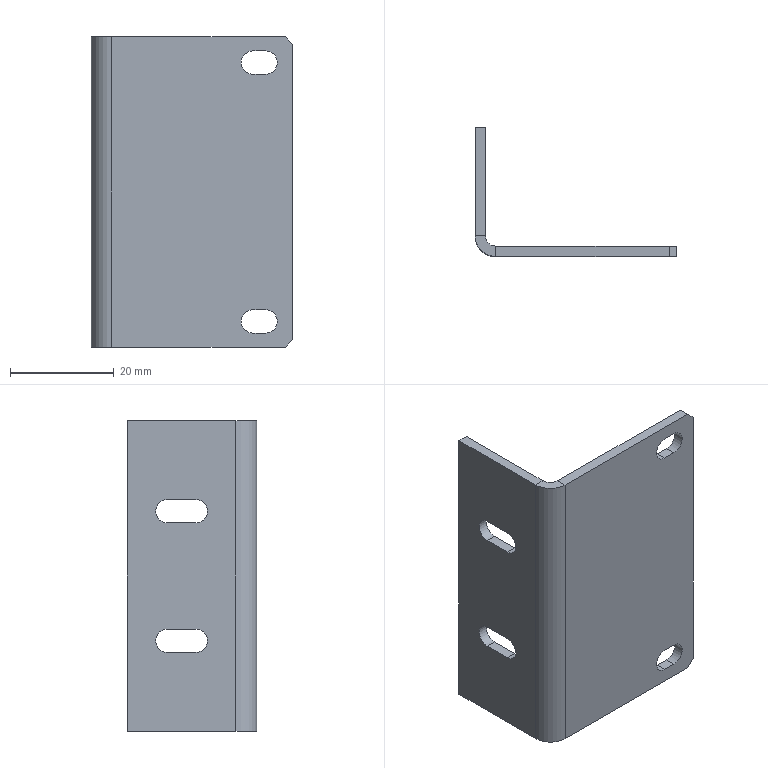Part | SolidWorks | features HoleWzd 2, Chamfer 1, FlatPattern 1, SMBaseFlange 1, SheetMetal 1 | 1 solid | 32 faces | box 39 x 25 x 60 mm | volume 7010 mm3 | plane 22 | cylinder 10 | commonest cylinder face diameters 4.5 x8 4 x1 8 x1
STEP:
#1=CARTESIAN_POINT('',(0.,-21.,60.));
#2=VERTEX_POINT('',#1);
#3=CARTESIAN_POINT('',(2.,-21.,60.));
#4=VERTEX_POINT('',#3);
#5=CARTESIAN_POINT('',(0.,-21.,60.));
#6=DIRECTION('',(1.,0.,0.));
#7=VECTOR('',#6,1000.);
#8=LINE('',#5,#7);
#9=EDGE_CURVE('',#2,#4,#8,.T.);
#10=ORIENTED_EDGE('',*,*,#9,.F.);
#11=CARTESIAN_POINT('',(4.,-25.,60.));
#12=VERTEX_POINT('',#11);
#13=CARTESIAN_POINT('',(4.,-21.,60.));
#14=DIRECTION('',(0.,0.,1.));
#15=DIRECTION('',(-1.,0.,0.));
#16=AXIS2_PLACEMENT_3D('',#13,#14,#15);
#17=CIRCLE('',#16,4.);
#18=EDGE_CURVE('',#2,#12,#17,.T.);
#19=ORIENTED_EDGE('',*,*,#18,.T.);
#20=CARTESIAN_POINT('',(4.,-23.,60.));
#21=VERTEX_POINT('',#20);
#22=CARTESIAN_POINT('',(4.,-23.,60.));
#23=DIRECTION('',(0.,-1.,0.));
#24=VECTOR('',#23,1000.);
#25=LINE('',#22,#24);
#26=EDGE_CURVE('',#21,#12,#25,.T.);
#27=ORIENTED_EDGE('',*,*,#26,.F.);
#28=CARTESIAN_POINT('',(4.,-21.,60.));
#29=DIRECTION('',(0.,0.,1.));
#30=DIRECTION('',(1.,0.,0.));
#31=AXIS2_PLACEMENT_3D('',#28,#29,#30);
#32=CIRCLE('',#31,2.);
#33=EDGE_CURVE('',#4,#21,#32,.T.);
#34=ORIENTED_EDGE('',*,*,#33,.F.);
#35=EDGE_LOOP('',(#10,#19,#27,#34));
#36=FACE_OUTER_BOUND('',#35,.T.);
#37=CARTESIAN_POINT('',(0.,-21.,60.));
#38=DIRECTION('',(0.,0.,1.));
#39=DIRECTION('',(1.,0.,0.));
#40=AXIS2_PLACEMENT_3D('',#37,#38,#39);
#41=PLANE('',#40);
#42=ADVANCED_FACE('',(#36),#41,.T.);
#43=CARTESIAN_POINT('',(0.,0.,60.));
#44=VERTEX_POINT('',#43);
#45=CARTESIAN_POINT('',(0.,0.,60.));
#46=DIRECTION('',(0.,-1.,0.));
#47=VECTOR('',#46,1000.);
#48=LINE('',#45,#47);
#49=EDGE_CURVE('',#44,#2,#48,.T.);
#50=ORIENTED_EDGE('',*,*,#49,.T.);
#51=ORIENTED_EDGE('',*,*,#9,.T.);
#52=CARTESIAN_POINT('',(2.,0.,60.));
#53=VERTEX_POINT('',#52);
#54=CARTESIAN_POINT('',(2.,0.,60.));
#55=DIRECTION('',(0.,-1.,0.));
#56=VECTOR('',#55,1000.);
#57=LINE('',#54,#56);
#58=EDGE_CURVE('',#53,#4,#57,.T.);
#59=ORIENTED_EDGE('',*,*,#58,.F.);
#60=CARTESIAN_POINT('',(0.,0.,60.));
#61=DIRECTION('',(1.,0.,0.));
#62=VECTOR('',#61,1000.);
#63=LINE('',#60,#62);
#64=EDGE_CURVE('',#44,#53,#63,.T.);
#65=ORIENTED_EDGE('',*,*,#64,.F.);
#66=EDGE_LOOP('',(#50,#51,#59,#65));
#67=FACE_OUTER_BOUND('',#66,.T.);
#68=CARTESIAN_POINT('',(4.,-23.,60.));
#69=DIRECTION('',(0.,0.,1.));
#70=DIRECTION('',(1.,0.,0.));
#71=AXIS2_PLACEMENT_3D('',#68,#69,#70);
#72=PLANE('',#71);
#73=ADVANCED_FACE('',(#67),#72,.T.);
#74=CARTESIAN_POINT('',(4.,-25.,0.));
#75=VERTEX_POINT('',#74);
#76=CARTESIAN_POINT('',(4.,-23.,0.));
#77=VERTEX_POINT('',#76);
#78=CARTESIAN_POINT('',(4.,-25.,0.));
#79=DIRECTION('',(0.,1.,0.));
#80=VECTOR('',#79,1000.);
#81=LINE('',#78,#80);
#82=EDGE_CURVE('',#75,#77,#81,.T.);
#83=ORIENTED_EDGE('',*,*,#82,.F.);
#84=CARTESIAN_POINT('',(0.,-21.,0.));
#85=VERTEX_POINT('',#84);
#86=CARTESIAN_POINT('',(4.,-21.,0.));
#87=DIRECTION('',(0.,0.,1.));
#88=DIRECTION('',(-1.,0.,0.));
#89=AXIS2_PLACEMENT_3D('',#86,#87,#88);
#90=CIRCLE('',#89,4.);
#91=EDGE_CURVE('',#85,#75,#90,.T.);
#92=ORIENTED_EDGE('',*,*,#91,.F.);
#93=CARTESIAN_POINT('',(2.,-21.,0.));
#94=VERTEX_POINT('',#93);
#95=CARTESIAN_POINT('',(2.,-21.,0.));
#96=DIRECTION('',(-1.,0.,0.));
#97=VECTOR('',#96,1000.);
#98=LINE('',#95,#97);
#99=EDGE_CURVE('',#94,#85,#98,.T.);
#100=ORIENTED_EDGE('',*,*,#99,.F.);
#101=CARTESIAN_POINT('',(4.,-21.,0.));
#102=DIRECTION('',(0.,0.,1.));
#103=DIRECTION('',(1.,0.,0.));
#104=AXIS2_PLACEMENT_3D('',#101,#102,#103);
#105=CIRCLE('',#104,2.);
#106=EDGE_CURVE('',#94,#77,#105,.T.);
#107=ORIENTED_EDGE('',*,*,#106,.T.);
#108=EDGE_LOOP('',(#83,#92,#100,#107));
#109=FACE_OUTER_BOUND('',#108,.T.);
#110=CARTESIAN_POINT('',(4.,-25.,0.));
#111=DIRECTION('',(0.,0.,-1.));
#112=DIRECTION('',(-1.,0.,0.));
#113=AXIS2_PLACEMENT_3D('',#110,#111,#112);
#114=PLANE('',#113);
#115=ADVANCED_FACE('',(#109),#114,.T.);
#116=CARTESIAN_POINT('',(37.5,-23.,0.));
#117=VERTEX_POINT('',#116);
#118=CARTESIAN_POINT('',(0.,-23.,0.));
#119=DIRECTION('',(1.,0.,0.));
#120=VECTOR('',#119,1000.);
#121=LINE('',#118,#120);
#122=EDGE_CURVE('',#77,#117,#121,.T.);
#123=ORIENTED_EDGE('',*,*,#122,.T.);
#124=CARTESIAN_POINT('',(37.5,-25.,0.));
#125=VERTEX_POINT('',#124);
#126=CARTESIAN_POINT('',(37.5,-21.,0.));
#127=DIRECTION('',(0.,-1.,0.));
#128=VECTOR('',#127,1000.);
#129=LINE('',#126,#128);
#130=EDGE_CURVE('',#117,#125,#129,.T.);
#131=ORIENTED_EDGE('',*,*,#130,.T.);
#132=CARTESIAN_POINT('',(0.,-25.,0.));
#133=DIRECTION('',(1.,0.,0.));
#134=VECTOR('',#133,1000.);
#135=LINE('',#132,#134);
#136=EDGE_CURVE('',#75,#125,#135,.T.);
#137=ORIENTED_EDGE('',*,*,#136,.F.);
#138=ORIENTED_EDGE('',*,*,#82,.T.);
#139=EDGE_LOOP('',(#123,#131,#137,#138));
#140=FACE_OUTER_BOUND('',#139,.T.);
#141=CARTESIAN_POINT('',(2.,-21.,0.));
#142=DIRECTION('',(0.,0.,-1.));
#143=DIRECTION('',(-1.,0.,0.));
#144=AXIS2_PLACEMENT_3D('',#141,#142,#143);
#145=PLANE('',#144);
#146=ADVANCED_FACE('',(#140),#145,.T.);
#147=CARTESIAN_POINT('',(33.75,-25.,2.75));
#148=VERTEX_POINT('',#147);
#149=CARTESIAN_POINT('',(31.25,-25.,2.75));
#150=VERTEX_POINT('',#149);
#151=CARTESIAN_POINT('',(0.,-25.,2.75));
#152=DIRECTION('',(-1.,0.,0.));
#153=VECTOR('',#152,1000.);
#154=LINE('',#151,#153);
#155=EDGE_CURVE('',#148,#150,#154,.T.);
#156=ORIENTED_EDGE('',*,*,#155,.T.);
#157=CARTESIAN_POINT('',(31.25,-25.,7.25));
#158=VERTEX_POINT('',#157);
#159=CARTESIAN_POINT('',(31.25,-25.,5.));
#160=DIRECTION('',(0.,1.,0.));
#161=DIRECTION('',(0.,0.,1.));
#162=AXIS2_PLACEMENT_3D('',#159,#160,#161);
#163=CIRCLE('',#162,2.25);
#164=EDGE_CURVE('',#150,#158,#163,.T.);
#165=ORIENTED_EDGE('',*,*,#164,.T.);
#166=CARTESIAN_POINT('',(33.75,-25.,7.25));
#167=VERTEX_POINT('',#166);
#168=CARTESIAN_POINT('',(0.,-25.,7.25));
#169=DIRECTION('',(1.,0.,0.));
#170=VECTOR('',#169,1000.);
#171=LINE('',#168,#170);
#172=EDGE_CURVE('',#158,#167,#171,.T.);
#173=ORIENTED_EDGE('',*,*,#172,.T.);
#174=CARTESIAN_POINT('',(33.75,-25.,5.));
#175=DIRECTION('',(0.,1.,0.));
#176=DIRECTION('',(0.,0.,1.));
#177=AXIS2_PLACEMENT_3D('',#174,#175,#176);
#178=CIRCLE('',#177,2.25);
#179=EDGE_CURVE('',#167,#148,#178,.T.);
#180=ORIENTED_EDGE('',*,*,#179,.T.);
#181=EDGE_LOOP('',(#156,#165,#173,#180));
#182=FACE_BOUND('',#181,.T.);
#183=CARTESIAN_POINT('',(33.75,-25.,57.25));
#184=VERTEX_POINT('',#183);
#185=CARTESIAN_POINT('',(33.75,-25.,52.75));
#186=VERTEX_POINT('',#185);
#187=CARTESIAN_POINT('',(33.75,-25.,55.));
#188=DIRECTION('',(0.,1.,0.));
#189=DIRECTION('',(0.,0.,1.));
#190=AXIS2_PLACEMENT_3D('',#187,#188,#189);
#191=CIRCLE('',#190,2.25);
#192=EDGE_CURVE('',#184,#186,#191,.T.);
#193=ORIENTED_EDGE('',*,*,#192,.T.);
#194=CARTESIAN_POINT('',(31.25,-25.,52.75));
#195=VERTEX_POINT('',#194);
#196=CARTESIAN_POINT('',(0.,-25.,52.75));
#197=DIRECTION('',(-1.,0.,0.));
#198=VECTOR('',#197,1000.);
#199=LINE('',#196,#198);
#200=EDGE_CURVE('',#186,#195,#199,.T.);
#201=ORIENTED_EDGE('',*,*,#200,.T.);
#202=CARTESIAN_POINT('',(31.25,-25.,57.25));
#203=VERTEX_POINT('',#202);
#204=CARTESIAN_POINT('',(31.25,-25.,55.));
#205=DIRECTION('',(0.,1.,0.));
#206=DIRECTION('',(0.,0.,1.));
#207=AXIS2_PLACEMENT_3D('',#204,#205,#206);
#208=CIRCLE('',#207,2.25);
#209=EDGE_CURVE('',#195,#203,#208,.T.);
#210=ORIENTED_EDGE('',*,*,#209,.T.);
#211=CARTESIAN_POINT('',(0.,-25.,57.25));
#212=DIRECTION('',(1.,0.,0.));
#213=VECTOR('',#212,1000.);
#214=LINE('',#211,#213);
#215=EDGE_CURVE('',#203,#184,#214,.T.);
#216=ORIENTED_EDGE('',*,*,#215,.T.);
#217=EDGE_LOOP('',(#193,#201,#210,#216));
#218=FACE_BOUND('',#217,.T.);
#219=CARTESIAN_POINT('',(39.,-25.,58.5));
#220=VERTEX_POINT('',#219);
#221=CARTESIAN_POINT('',(39.,-25.,1.5));
#222=VERTEX_POINT('',#221);
#223=CARTESIAN_POINT('',(39.,-25.,60.));
#224=DIRECTION('',(0.,0.,-1.));
#225=VECTOR('',#224,1000.);
#226=LINE('',#223,#225);
#227=EDGE_CURVE('',#220,#222,#226,.T.);
#228=ORIENTED_EDGE('',*,*,#227,.F.);
#229=CARTESIAN_POINT('',(37.5,-25.,60.));
#230=VERTEX_POINT('',#229);
#231=CARTESIAN_POINT('',(39.,-25.,58.5));
#232=DIRECTION('',(-0.7071,0.,0.7071));
#233=VECTOR('',#232,1000.);
#234=LINE('',#231,#233);
#235=EDGE_CURVE('',#220,#230,#234,.T.);
#236=ORIENTED_EDGE('',*,*,#235,.T.);
#237=CARTESIAN_POINT('',(0.,-25.,60.));
#238=DIRECTION('',(1.,0.,0.));
#239=VECTOR('',#238,1000.);
#240=LINE('',#237,#239);
#241=EDGE_CURVE('',#12,#230,#240,.T.);
#242=ORIENTED_EDGE('',*,*,#241,.F.);
#243=CARTESIAN_POINT('',(4.,-25.,60.));
#244=DIRECTION('',(0.,0.,-1.));
#245=VECTOR('',#244,1000.);
#246=LINE('',#243,#245);
#247=EDGE_CURVE('',#12,#75,#246,.T.);
#248=ORIENTED_EDGE('',*,*,#247,.T.);
#249=ORIENTED_EDGE('',*,*,#136,.T.);
#250=CARTESIAN_POINT('',(37.5,-25.,0.));
#251=DIRECTION('',(0.7071,0.,0.7071));
#252=VECTOR('',#251,1000.);
#253=LINE('',#250,#252);
#254=EDGE_CURVE('',#125,#222,#253,.T.);
#255=ORIENTED_EDGE('',*,*,#254,.T.);
#256=EDGE_LOOP('',(#228,#236,#242,#248,#249,#255));
#257=FACE_OUTER_BOUND('',#256,.T.);
#258=CARTESIAN_POINT('',(0.,-25.,60.));
#259=DIRECTION('',(0.,1.,0.));
#260=DIRECTION('',(0.,0.,1.));
#261=AXIS2_PLACEMENT_3D('',#258,#259,#260);
#262=PLANE('',#261);
#263=ADVANCED_FACE('',(#182,#218,#257),#262,.F.);
#264=CARTESIAN_POINT('',(39.,-23.,58.5));
#265=VERTEX_POINT('',#264);
#266=CARTESIAN_POINT('',(39.,-23.,1.5));
#267=VERTEX_POINT('',#266);
#268=CARTESIAN_POINT('',(39.,-23.,60.));
#269=DIRECTION('',(0.,0.,-1.));
#270=VECTOR('',#269,1000.);
#271=LINE('',#268,#270);
#272=EDGE_CURVE('',#265,#267,#271,.T.);
#273=ORIENTED_EDGE('',*,*,#272,.F.);
#274=CARTESIAN_POINT('',(39.,-23.,58.5));
#275=DIRECTION('',(0.,-1.,0.));
#276=VECTOR('',#275,1000.);
#277=LINE('',#274,#276);
#278=EDGE_CURVE('',#265,#220,#277,.T.);
#279=ORIENTED_EDGE('',*,*,#278,.T.);
#280=ORIENTED_EDGE('',*,*,#227,.T.);
#281=CARTESIAN_POINT('',(39.,-23.,1.5));
#282=DIRECTION('',(0.,1.,0.));
#283=VECTOR('',#282,1000.);
#284=LINE('',#281,#283);
#285=EDGE_CURVE('',#222,#267,#284,.T.);
#286=ORIENTED_EDGE('',*,*,#285,.T.);
#287=EDGE_LOOP('',(#273,#279,#280,#286));
#288=FACE_OUTER_BOUND('',#287,.T.);
#289=CARTESIAN_POINT('',(39.,-23.,60.));
#290=DIRECTION('',(1.,0.,0.));
#291=DIRECTION('',(0.,0.,-1.));
#292=AXIS2_PLACEMENT_3D('',#289,#290,#291);
#293=PLANE('',#292);
#294=ADVANCED_FACE('',(#288),#293,.T.);
#295=CARTESIAN_POINT('',(31.25,-23.,7.25));
#296=VERTEX_POINT('',#295);
#297=CARTESIAN_POINT('',(33.75,-23.,7.25));
#298=VERTEX_POINT('',#297);
#299=CARTESIAN_POINT('',(31.25,-23.,7.25));
#300=DIRECTION('',(1.,0.,0.));
#301=VECTOR('',#300,1000.);
#302=LINE('',#299,#301);
#303=EDGE_CURVE('',#296,#298,#302,.T.);
#304=ORIENTED_EDGE('',*,*,#303,.F.);
#305=CARTESIAN_POINT('',(31.25,-23.,2.75));
#306=VERTEX_POINT('',#305);
#307=CARTESIAN_POINT('',(31.25,-23.,5.));
#308=DIRECTION('',(0.,1.,0.));
#309=DIRECTION('',(0.,0.,1.));
#310=AXIS2_PLACEMENT_3D('',#307,#308,#309);
#311=CIRCLE('',#310,2.25);
#312=EDGE_CURVE('',#306,#296,#311,.T.);
#313=ORIENTED_EDGE('',*,*,#312,.F.);
#314=CARTESIAN_POINT('',(33.75,-23.,2.75));
#315=VERTEX_POINT('',#314);
#316=CARTESIAN_POINT('',(31.25,-23.,2.75));
#317=DIRECTION('',(1.,0.,0.));
#318=VECTOR('',#317,1000.);
#319=LINE('',#316,#318);
#320=EDGE_CURVE('',#306,#315,#319,.T.);
#321=ORIENTED_EDGE('',*,*,#320,.T.);
#322=CARTESIAN_POINT('',(33.75,-23.,5.));
#323=DIRECTION('',(0.,1.,0.));
#324=DIRECTION('',(0.,0.,1.));
#325=AXIS2_PLACEMENT_3D('',#322,#323,#324);
#326=CIRCLE('',#325,2.25);
#327=EDGE_CURVE('',#298,#315,#326,.T.);
#328=ORIENTED_EDGE('',*,*,#327,.F.);
#329=EDGE_LOOP('',(#304,#313,#321,#328));
#330=FACE_BOUND('',#329,.T.);
#331=CARTESIAN_POINT('',(33.75,-23.,57.25));
#332=VERTEX_POINT('',#331);
#333=CARTESIAN_POINT('',(33.75,-23.,52.75));
#334=VERTEX_POINT('',#333);
#335=CARTESIAN_POINT('',(33.75,-23.,55.));
#336=DIRECTION('',(0.,1.,0.));
#337=DIRECTION('',(0.,0.,1.));
#338=AXIS2_PLACEMENT_3D('',#335,#336,#337);
#339=CIRCLE('',#338,2.25);
#340=EDGE_CURVE('',#332,#334,#339,.T.);
#341=ORIENTED_EDGE('',*,*,#340,.F.);
#342=CARTESIAN_POINT('',(31.25,-23.,57.25));
#343=VERTEX_POINT('',#342);
#344=CARTESIAN_POINT('',(31.25,-23.,57.25));
#345=DIRECTION('',(1.,0.,0.));
#346=VECTOR('',#345,1000.);
#347=LINE('',#344,#346);
#348=EDGE_CURVE('',#343,#332,#347,.T.);
#349=ORIENTED_EDGE('',*,*,#348,.F.);
#350=CARTESIAN_POINT('',(31.25,-23.,52.75));
#351=VERTEX_POINT('',#350);
#352=CARTESIAN_POINT('',(31.25,-23.,55.));
#353=DIRECTION('',(0.,1.,0.));
#354=DIRECTION('',(0.,0.,1.));
#355=AXIS2_PLACEMENT_3D('',#352,#353,#354);
#356=CIRCLE('',#355,2.25);
#357=EDGE_CURVE('',#351,#343,#356,.T.);
#358=ORIENTED_EDGE('',*,*,#357,.F.);
#359=CARTESIAN_POINT('',(31.25,-23.,52.75));
#360=DIRECTION('',(1.,0.,0.));
#361=VECTOR('',#360,1000.);
#362=LINE('',#359,#361);
#363=EDGE_CURVE('',#351,#334,#362,.T.);
#364=ORIENTED_EDGE('',*,*,#363,.T.);
#365=EDGE_LOOP('',(#341,#349,#358,#364));
#366=FACE_BOUND('',#365,.T.);
#367=CARTESIAN_POINT('',(37.5,-23.,60.));
#368=VERTEX_POINT('',#367);
#369=CARTESIAN_POINT('',(0.,-23.,60.));
#370=DIRECTION('',(1.,0.,0.));
#371=VECTOR('',#370,1000.);
#372=LINE('',#369,#371);
#373=EDGE_CURVE('',#21,#368,#372,.T.);
#374=ORIENTED_EDGE('',*,*,#373,.T.);
#375=CARTESIAN_POINT('',(18.75,-23.,78.75));
#376=DIRECTION('',(0.7071,0.,-0.7071));
#377=VECTOR('',#376,1000.);
#378=LINE('',#375,#377);
#379=EDGE_CURVE('',#368,#265,#378,.T.);
#380=ORIENTED_EDGE('',*,*,#379,.T.);
#381=ORIENTED_EDGE('',*,*,#272,.T.);
#382=CARTESIAN_POINT('',(48.75,-23.,11.25));
#383=DIRECTION('',(-0.7071,0.,-0.7071));
#384=VECTOR('',#383,1000.);
#385=LINE('',#382,#384);
#386=EDGE_CURVE('',#267,#117,#385,.T.);
#387=ORIENTED_EDGE('',*,*,#386,.T.);
#388=ORIENTED_EDGE('',*,*,#122,.F.);
#389=CARTESIAN_POINT('',(4.,-23.,60.));
#390=DIRECTION('',(0.,0.,-1.));
#391=VECTOR('',#390,1000.);
#392=LINE('',#389,#391);
#393=EDGE_CURVE('',#21,#77,#392,.T.);
#394=ORIENTED_EDGE('',*,*,#393,.F.);
#395=EDGE_LOOP('',(#374,#380,#381,#387,#388,#394));
#396=FACE_OUTER_BOUND('',#395,.T.);
#397=CARTESIAN_POINT('',(0.,-23.,60.));
#398=DIRECTION('',(0.,1.,0.));
#399=DIRECTION('',(0.,0.,1.));
#400=AXIS2_PLACEMENT_3D('',#397,#398,#399);
#401=PLANE('',#400);
#402=ADVANCED_FACE('',(#330,#366,#396),#401,.T.);
#403=ORIENTED_EDGE('',*,*,#106,.F.);
#404=CARTESIAN_POINT('',(2.,-21.,60.));
#405=DIRECTION('',(0.,0.,-1.));
#406=VECTOR('',#405,1000.);
#407=LINE('',#404,#406);
#408=EDGE_CURVE('',#4,#94,#407,.T.);
#409=ORIENTED_EDGE('',*,*,#408,.F.);
#410=ORIENTED_EDGE('',*,*,#33,.T.);
#411=ORIENTED_EDGE('',*,*,#393,.T.);
#412=EDGE_LOOP('',(#403,#409,#410,#411));
#413=FACE_OUTER_BOUND('',#412,.T.);
#414=CARTESIAN_POINT('',(4.,-21.,60.));
#415=DIRECTION('',(0.,0.,-1.));
#416=DIRECTION('',(-1.,0.,0.));
#417=AXIS2_PLACEMENT_3D('',#414,#415,#416);
#418=CYLINDRICAL_SURFACE('',#417,2.);
#419=ADVANCED_FACE('',(#413),#418,.F.);
#420=CARTESIAN_POINT('',(2.,-7.75,40.25));
#421=VERTEX_POINT('',#420);
#422=CARTESIAN_POINT('',(2.,-7.75,44.75));
#423=VERTEX_POINT('',#422);
#424=CARTESIAN_POINT('',(2.,-7.75,42.5));
#425=DIRECTION('',(1.,0.,0.));
#426=DIRECTION('',(0.,0.,-1.));
#427=AXIS2_PLACEMENT_3D('',#424,#425,#426);
#428=CIRCLE('',#427,2.25);
#429=EDGE_CURVE('',#421,#423,#428,.T.);
#430=ORIENTED_EDGE('',*,*,#429,.F.);
#431=CARTESIAN_POINT('',(2.,-13.25,40.25));
#432=VERTEX_POINT('',#431);
#433=CARTESIAN_POINT('',(2.,-13.25,40.25));
#434=DIRECTION('',(0.,1.,0.));
#435=VECTOR('',#434,1000.);
#436=LINE('',#433,#435);
#437=EDGE_CURVE('',#432,#421,#436,.T.);
#438=ORIENTED_EDGE('',*,*,#437,.F.);
#439=CARTESIAN_POINT('',(2.,-13.25,44.75));
#440=VERTEX_POINT('',#439);
#441=CARTESIAN_POINT('',(2.,-13.25,42.5));
#442=DIRECTION('',(1.,0.,0.));
#443=DIRECTION('',(0.,0.,-1.));
#444=AXIS2_PLACEMENT_3D('',#441,#442,#443);
#445=CIRCLE('',#444,2.25);
#446=EDGE_CURVE('',#440,#432,#445,.T.);
#447=ORIENTED_EDGE('',*,*,#446,.F.);
#448=CARTESIAN_POINT('',(2.,-13.25,44.75));
#449=DIRECTION('',(0.,1.,0.));
#450=VECTOR('',#449,1000.);
#451=LINE('',#448,#450);
#452=EDGE_CURVE('',#440,#423,#451,.T.);
#453=ORIENTED_EDGE('',*,*,#452,.T.);
#454=EDGE_LOOP('',(#430,#438,#447,#453));
#455=FACE_BOUND('',#454,.T.);
#456=CARTESIAN_POINT('',(2.,-7.75,15.25));
#457=VERTEX_POINT('',#456);
#458=CARTESIAN_POINT('',(2.,-7.75,19.75));
#459=VERTEX_POINT('',#458);
#460=CARTESIAN_POINT('',(2.,-7.75,17.5));
#461=DIRECTION('',(1.,0.,0.));
#462=DIRECTION('',(0.,0.,-1.));
#463=AXIS2_PLACEMENT_3D('',#460,#461,#462);
#464=CIRCLE('',#463,2.25);
#465=EDGE_CURVE('',#457,#459,#464,.T.);
#466=ORIENTED_EDGE('',*,*,#465,.F.);
#467=CARTESIAN_POINT('',(2.,-13.25,15.25));
#468=VERTEX_POINT('',#467);
#469=CARTESIAN_POINT('',(2.,-13.25,15.25));
#470=DIRECTION('',(0.,1.,0.));
#471=VECTOR('',#470,1000.);
#472=LINE('',#469,#471);
#473=EDGE_CURVE('',#468,#457,#472,.T.);
#474=ORIENTED_EDGE('',*,*,#473,.F.);
#475=CARTESIAN_POINT('',(2.,-13.25,19.75));
#476=VERTEX_POINT('',#475);
#477=CARTESIAN_POINT('',(2.,-13.25,17.5));
#478=DIRECTION('',(1.,0.,0.));
#479=DIRECTION('',(0.,0.,-1.));
#480=AXIS2_PLACEMENT_3D('',#477,#478,#479);
#481=CIRCLE('',#480,2.25);
#482=EDGE_CURVE('',#476,#468,#481,.T.);
#483=ORIENTED_EDGE('',*,*,#482,.F.);
#484=CARTESIAN_POINT('',(2.,-13.25,19.75));
#485=DIRECTION('',(0.,1.,0.));
#486=VECTOR('',#485,1000.);
#487=LINE('',#484,#486);
#488=EDGE_CURVE('',#476,#459,#487,.T.);
#489=ORIENTED_EDGE('',*,*,#488,.T.);
#490=EDGE_LOOP('',(#466,#474,#483,#489));
#491=FACE_BOUND('',#490,.T.);
#492=CARTESIAN_POINT('',(2.,0.,0.));
#493=VERTEX_POINT('',#492);
#494=CARTESIAN_POINT('',(2.,0.,0.));
#495=DIRECTION('',(0.,-1.,0.));
#496=VECTOR('',#495,1000.);
#497=LINE('',#494,#496);
#498=EDGE_CURVE('',#493,#94,#497,.T.);
#499=ORIENTED_EDGE('',*,*,#498,.F.);
#500=CARTESIAN_POINT('',(2.,0.,60.));
#501=DIRECTION('',(0.,0.,-1.));
#502=VECTOR('',#501,1000.);
#503=LINE('',#500,#502);
#504=EDGE_CURVE('',#53,#493,#503,.T.);
#505=ORIENTED_EDGE('',*,*,#504,.F.);
#506=ORIENTED_EDGE('',*,*,#58,.T.);
#507=ORIENTED_EDGE('',*,*,#408,.T.);
#508=EDGE_LOOP('',(#499,#505,#506,#507));
#509=FACE_OUTER_BOUND('',#508,.T.);
#510=CARTESIAN_POINT('',(2.,0.,60.));
#511=DIRECTION('',(1.,0.,0.));
#512=DIRECTION('',(0.,1.,0.));
#513=AXIS2_PLACEMENT_3D('',#510,#511,#512);
#514=PLANE('',#513);
#515=ADVANCED_FACE('',(#455,#491,#509),#514,.T.);
#516=CARTESIAN_POINT('',(0.,0.,0.));
#517=VERTEX_POINT('',#516);
#518=CARTESIAN_POINT('',(0.,0.,0.));
#519=DIRECTION('',(1.,0.,0.));
#520=VECTOR('',#519,1000.);
#521=LINE('',#518,#520);
#522=EDGE_CURVE('',#517,#493,#521,.T.);
#523=ORIENTED_EDGE('',*,*,#522,.F.);
#524=CARTESIAN_POINT('',(0.,0.,60.));
#525=DIRECTION('',(0.,0.,-1.));
#526=VECTOR('',#525,1000.);
#527=LINE('',#524,#526);
#528=EDGE_CURVE('',#44,#517,#527,.T.);
#529=ORIENTED_EDGE('',*,*,#528,.F.);
#530=ORIENTED_EDGE('',*,*,#64,.T.);
#531=ORIENTED_EDGE('',*,*,#504,.T.);
#532=EDGE_LOOP('',(#523,#529,#530,#531));
#533=FACE_OUTER_BOUND('',#532,.T.);
#534=CARTESIAN_POINT('',(0.,0.,60.));
#535=DIRECTION('',(0.,1.,0.));
#536=DIRECTION('',(-1.,0.,0.));
#537=AXIS2_PLACEMENT_3D('',#534,#535,#536);
#538=PLANE('',#537);
#539=ADVANCED_FACE('',(#533),#538,.T.);
#540=CARTESIAN_POINT('',(0.,-13.25,44.75));
#541=VERTEX_POINT('',#540);
#542=CARTESIAN_POINT('',(0.,-13.25,40.25));
#543=VERTEX_POINT('',#542);
#544=CARTESIAN_POINT('',(0.,-13.25,42.5));
#545=DIRECTION('',(1.,0.,0.));
#546=DIRECTION('',(0.,1.,0.));
#547=AXIS2_PLACEMENT_3D('',#544,#545,#546);
#548=CIRCLE('',#547,2.25);
#549=EDGE_CURVE('',#541,#543,#548,.T.);
#550=ORIENTED_EDGE('',*,*,#549,.T.);
#551=CARTESIAN_POINT('',(0.,-7.75,40.25));
#552=VERTEX_POINT('',#551);
#553=CARTESIAN_POINT('',(0.,0.,40.25));
#554=DIRECTION('',(0.,1.,0.));
#555=VECTOR('',#554,1000.);
#556=LINE('',#553,#555);
#557=EDGE_CURVE('',#543,#552,#556,.T.);
#558=ORIENTED_EDGE('',*,*,#557,.T.);
#559=CARTESIAN_POINT('',(0.,-7.75,44.75));
#560=VERTEX_POINT('',#559);
#561=CARTESIAN_POINT('',(0.,-7.75,42.5));
#562=DIRECTION('',(1.,0.,0.));
#563=DIRECTION('',(0.,1.,0.));
#564=AXIS2_PLACEMENT_3D('',#561,#562,#563);
#565=CIRCLE('',#564,2.25);
#566=EDGE_CURVE('',#552,#560,#565,.T.);
#567=ORIENTED_EDGE('',*,*,#566,.T.);
#568=CARTESIAN_POINT('',(0.,0.,44.75));
#569=DIRECTION('',(0.,-1.,0.));
#570=VECTOR('',#569,1000.);
#571=LINE('',#568,#570);
#572=EDGE_CURVE('',#560,#541,#571,.T.);
#573=ORIENTED_EDGE('',*,*,#572,.T.);
#574=EDGE_LOOP('',(#550,#558,#567,#573));
#575=FACE_BOUND('',#574,.T.);
#576=CARTESIAN_POINT('',(0.,-13.25,19.75));
#577=VERTEX_POINT('',#576);
#578=CARTESIAN_POINT('',(0.,-13.25,15.25));
#579=VERTEX_POINT('',#578);
#580=CARTESIAN_POINT('',(0.,-13.25,17.5));
#581=DIRECTION('',(1.,0.,0.));
#582=DIRECTION('',(0.,1.,0.));
#583=AXIS2_PLACEMENT_3D('',#580,#581,#582);
#584=CIRCLE('',#583,2.25);
#585=EDGE_CURVE('',#577,#579,#584,.T.);
#586=ORIENTED_EDGE('',*,*,#585,.T.);
#587=CARTESIAN_POINT('',(0.,-7.75,15.25));
#588=VERTEX_POINT('',#587);
#589=CARTESIAN_POINT('',(0.,0.,15.25));
#590=DIRECTION('',(0.,1.,0.));
#591=VECTOR('',#590,1000.);
#592=LINE('',#589,#591);
#593=EDGE_CURVE('',#579,#588,#592,.T.);
#594=ORIENTED_EDGE('',*,*,#593,.T.);
#595=CARTESIAN_POINT('',(0.,-7.75,19.75));
#596=VERTEX_POINT('',#595);
#597=CARTESIAN_POINT('',(0.,-7.75,17.5));
#598=DIRECTION('',(1.,0.,0.));
#599=DIRECTION('',(0.,1.,0.));
#600=AXIS2_PLACEMENT_3D('',#597,#598,#599);
#601=CIRCLE('',#600,2.25);
#602=EDGE_CURVE('',#588,#596,#601,.T.);
#603=ORIENTED_EDGE('',*,*,#602,.T.);
#604=CARTESIAN_POINT('',(0.,0.,19.75));
#605=DIRECTION('',(0.,-1.,0.));
#606=VECTOR('',#605,1000.);
#607=LINE('',#604,#606);
#608=EDGE_CURVE('',#596,#577,#607,.T.);
#609=ORIENTED_EDGE('',*,*,#608,.T.);
#610=EDGE_LOOP('',(#586,#594,#603,#609));
#611=FACE_BOUND('',#610,.T.);
#612=CARTESIAN_POINT('',(0.,0.,0.));
#613=DIRECTION('',(0.,-1.,0.));
#614=VECTOR('',#613,1000.);
#615=LINE('',#612,#614);
#616=EDGE_CURVE('',#517,#85,#615,.T.);
#617=ORIENTED_EDGE('',*,*,#616,.T.);
#618=CARTESIAN_POINT('',(0.,-21.,60.));
#619=DIRECTION('',(0.,0.,-1.));
#620=VECTOR('',#619,1000.);
#621=LINE('',#618,#620);
#622=EDGE_CURVE('',#2,#85,#621,.T.);
#623=ORIENTED_EDGE('',*,*,#622,.F.);
#624=ORIENTED_EDGE('',*,*,#49,.F.);
#625=ORIENTED_EDGE('',*,*,#528,.T.);
#626=EDGE_LOOP('',(#617,#623,#624,#625));
#627=FACE_OUTER_BOUND('',#626,.T.);
#628=CARTESIAN_POINT('',(0.,0.,60.));
#629=DIRECTION('',(1.,0.,0.));
#630=DIRECTION('',(0.,1.,0.));
#631=AXIS2_PLACEMENT_3D('',#628,#629,#630);
#632=PLANE('',#631);
#633=ADVANCED_FACE('',(#575,#611,#627),#632,.F.);
#634=ORIENTED_EDGE('',*,*,#91,.T.);
#635=ORIENTED_EDGE('',*,*,#247,.F.);
#636=ORIENTED_EDGE('',*,*,#18,.F.);
#637=ORIENTED_EDGE('',*,*,#622,.T.);
#638=EDGE_LOOP('',(#634,#635,#636,#637));
#639=FACE_OUTER_BOUND('',#638,.T.);
#640=CARTESIAN_POINT('',(4.,-21.,60.));
#641=DIRECTION('',(0.,0.,-1.));
#642=DIRECTION('',(-1.,0.,0.));
#643=AXIS2_PLACEMENT_3D('',#640,#641,#642);
#644=CYLINDRICAL_SURFACE('',#643,4.);
#645=ADVANCED_FACE('',(#639),#644,.T.);
#646=ORIENTED_EDGE('',*,*,#241,.T.);
#647=CARTESIAN_POINT('',(37.5,-21.,60.));
#648=DIRECTION('',(0.,1.,0.));
#649=VECTOR('',#648,1000.);
#650=LINE('',#647,#649);
#651=EDGE_CURVE('',#230,#368,#650,.T.);
#652=ORIENTED_EDGE('',*,*,#651,.T.);
#653=ORIENTED_EDGE('',*,*,#373,.F.);
#654=ORIENTED_EDGE('',*,*,#26,.T.);
#655=EDGE_LOOP('',(#646,#652,#653,#654));
#656=FACE_OUTER_BOUND('',#655,.T.);
#657=CARTESIAN_POINT('',(4.,-21.,60.));
#658=DIRECTION('',(0.,0.,1.));
#659=DIRECTION('',(1.,0.,0.));
#660=AXIS2_PLACEMENT_3D('',#657,#658,#659);
#661=PLANE('',#660);
#662=ADVANCED_FACE('',(#656),#661,.T.);
#663=ORIENTED_EDGE('',*,*,#498,.T.);
#664=ORIENTED_EDGE('',*,*,#99,.T.);
#665=ORIENTED_EDGE('',*,*,#616,.F.);
#666=ORIENTED_EDGE('',*,*,#522,.T.);
#667=EDGE_LOOP('',(#663,#664,#665,#666));
#668=FACE_OUTER_BOUND('',#667,.T.);
#669=CARTESIAN_POINT('',(4.,-21.,0.));
#670=DIRECTION('',(0.,0.,1.));
#671=DIRECTION('',(1.,0.,0.));
#672=AXIS2_PLACEMENT_3D('',#669,#670,#671);
#673=PLANE('',#672);
#674=ADVANCED_FACE('',(#668),#673,.F.);
#675=CARTESIAN_POINT('',(31.25,-23.,52.75));
#676=DIRECTION('',(0.,-1.,0.));
#677=VECTOR('',#676,1000.);
#678=LINE('',#675,#677);
#679=EDGE_CURVE('',#351,#195,#678,.T.);
#680=ORIENTED_EDGE('',*,*,#679,.F.);
#681=ORIENTED_EDGE('',*,*,#357,.T.);
#682=CARTESIAN_POINT('',(31.25,-23.,57.25));
#683=DIRECTION('',(0.,1.,0.));
#684=VECTOR('',#683,1000.);
#685=LINE('',#682,#684);
#686=EDGE_CURVE('',#203,#343,#685,.T.);
#687=ORIENTED_EDGE('',*,*,#686,.F.);
#688=ORIENTED_EDGE('',*,*,#209,.F.);
#689=EDGE_LOOP('',(#680,#681,#687,#688));
#690=FACE_OUTER_BOUND('',#689,.T.);
#691=CARTESIAN_POINT('',(31.25,-23.,55.));
#692=DIRECTION('',(0.,1.,0.));
#693=DIRECTION('',(0.,0.,1.));
#694=AXIS2_PLACEMENT_3D('',#691,#692,#693);
#695=CYLINDRICAL_SURFACE('',#694,2.25);
#696=ADVANCED_FACE('',(#690),#695,.F.);
#697=ORIENTED_EDGE('',*,*,#686,.T.);
#698=ORIENTED_EDGE('',*,*,#348,.T.);
#699=CARTESIAN_POINT('',(33.75,-23.,57.25));
#700=DIRECTION('',(0.,-1.,0.));
#701=VECTOR('',#700,1000.);
#702=LINE('',#699,#701);
#703=EDGE_CURVE('',#332,#184,#702,.T.);
#704=ORIENTED_EDGE('',*,*,#703,.T.);
#705=ORIENTED_EDGE('',*,*,#215,.F.);
#706=EDGE_LOOP('',(#697,#698,#704,#705));
#707=FACE_OUTER_BOUND('',#706,.T.);
#708=CARTESIAN_POINT('',(31.25,-23.,57.25));
#709=DIRECTION('',(0.,0.,1.));
#710=DIRECTION('',(1.,0.,0.));
#711=AXIS2_PLACEMENT_3D('',#708,#709,#710);
#712=PLANE('',#711);
#713=ADVANCED_FACE('',(#707),#712,.F.);
#714=CARTESIAN_POINT('',(33.75,-23.,52.75));
#715=DIRECTION('',(0.,1.,0.));
#716=VECTOR('',#715,1000.);
#717=LINE('',#714,#716);
#718=EDGE_CURVE('',#186,#334,#717,.T.);
#719=ORIENTED_EDGE('',*,*,#718,.T.);
#720=ORIENTED_EDGE('',*,*,#363,.F.);
#721=ORIENTED_EDGE('',*,*,#679,.T.);
#722=ORIENTED_EDGE('',*,*,#200,.F.);
#723=EDGE_LOOP('',(#719,#720,#721,#722));
#724=FACE_OUTER_BOUND('',#723,.T.);
#725=CARTESIAN_POINT('',(31.25,-23.,52.75));
#726=DIRECTION('',(0.,0.,-1.));
#727=DIRECTION('',(-1.,0.,0.));
#728=AXIS2_PLACEMENT_3D('',#725,#726,#727);
#729=PLANE('',#728);
#730=ADVANCED_FACE('',(#724),#729,.F.);
#731=ORIENTED_EDGE('',*,*,#703,.F.);
#732=ORIENTED_EDGE('',*,*,#340,.T.);
#733=ORIENTED_EDGE('',*,*,#718,.F.);
#734=ORIENTED_EDGE('',*,*,#192,.F.);
#735=EDGE_LOOP('',(#731,#732,#733,#734));
#736=FACE_OUTER_BOUND('',#735,.T.);
#737=CARTESIAN_POINT('',(33.75,-23.,55.));
#738=DIRECTION('',(0.,1.,0.));
#739=DIRECTION('',(0.,0.,1.));
#740=AXIS2_PLACEMENT_3D('',#737,#738,#739);
#741=CYLINDRICAL_SURFACE('',#740,2.25);
#742=ADVANCED_FACE('',(#736),#741,.F.);
#743=CARTESIAN_POINT('',(33.75,-23.,2.75));
#744=DIRECTION('',(0.,1.,0.));
#745=VECTOR('',#744,1000.);
#746=LINE('',#743,#745);
#747=EDGE_CURVE('',#148,#315,#746,.T.);
#748=ORIENTED_EDGE('',*,*,#747,.T.);
#749=ORIENTED_EDGE('',*,*,#320,.F.);
#750=CARTESIAN_POINT('',(31.25,-23.,2.75));
#751=DIRECTION('',(0.,-1.,0.));
#752=VECTOR('',#751,1000.);
#753=LINE('',#750,#752);
#754=EDGE_CURVE('',#306,#150,#753,.T.);
#755=ORIENTED_EDGE('',*,*,#754,.T.);
#756=ORIENTED_EDGE('',*,*,#155,.F.);
#757=EDGE_LOOP('',(#748,#749,#755,#756));
#758=FACE_OUTER_BOUND('',#757,.T.);
#759=CARTESIAN_POINT('',(31.25,-23.,2.75));
#760=DIRECTION('',(0.,0.,-1.));
#761=DIRECTION('',(-1.,0.,0.));
#762=AXIS2_PLACEMENT_3D('',#759,#760,#761);
#763=PLANE('',#762);
#764=ADVANCED_FACE('',(#758),#763,.F.);
#765=ORIENTED_EDGE('',*,*,#754,.F.);
#766=ORIENTED_EDGE('',*,*,#312,.T.);
#767=CARTESIAN_POINT('',(31.25,-23.,7.25));
#768=DIRECTION('',(0.,1.,0.));
#769=VECTOR('',#768,1000.);
#770=LINE('',#767,#769);
#771=EDGE_CURVE('',#158,#296,#770,.T.);
#772=ORIENTED_EDGE('',*,*,#771,.F.);
#773=ORIENTED_EDGE('',*,*,#164,.F.);
#774=EDGE_LOOP('',(#765,#766,#772,#773));
#775=FACE_OUTER_BOUND('',#774,.T.);
#776=CARTESIAN_POINT('',(31.25,-23.,5.));
#777=DIRECTION('',(0.,1.,0.));
#778=DIRECTION('',(0.,0.,1.));
#779=AXIS2_PLACEMENT_3D('',#776,#777,#778);
#780=CYLINDRICAL_SURFACE('',#779,2.25);
#781=ADVANCED_FACE('',(#775),#780,.F.);
#782=ORIENTED_EDGE('',*,*,#771,.T.);
#783=ORIENTED_EDGE('',*,*,#303,.T.);
#784=CARTESIAN_POINT('',(33.75,-23.,7.25));
#785=DIRECTION('',(0.,-1.,0.));
#786=VECTOR('',#785,1000.);
#787=LINE('',#784,#786);
#788=EDGE_CURVE('',#298,#167,#787,.T.);
#789=ORIENTED_EDGE('',*,*,#788,.T.);
#790=ORIENTED_EDGE('',*,*,#172,.F.);
#791=EDGE_LOOP('',(#782,#783,#789,#790));
#792=FACE_OUTER_BOUND('',#791,.T.);
#793=CARTESIAN_POINT('',(31.25,-23.,7.25));
#794=DIRECTION('',(0.,0.,1.));
#795=DIRECTION('',(1.,0.,0.));
#796=AXIS2_PLACEMENT_3D('',#793,#794,#795);
#797=PLANE('',#796);
#798=ADVANCED_FACE('',(#792),#797,.F.);
#799=ORIENTED_EDGE('',*,*,#788,.F.);
#800=ORIENTED_EDGE('',*,*,#327,.T.);
#801=ORIENTED_EDGE('',*,*,#747,.F.);
#802=ORIENTED_EDGE('',*,*,#179,.F.);
#803=EDGE_LOOP('',(#799,#800,#801,#802));
#804=FACE_OUTER_BOUND('',#803,.T.);
#805=CARTESIAN_POINT('',(33.75,-23.,5.));
#806=DIRECTION('',(0.,1.,0.));
#807=DIRECTION('',(0.,0.,1.));
#808=AXIS2_PLACEMENT_3D('',#805,#806,#807);
#809=CYLINDRICAL_SURFACE('',#808,2.25);
#810=ADVANCED_FACE('',(#804),#809,.F.);
#811=ORIENTED_EDGE('',*,*,#379,.F.);
#812=ORIENTED_EDGE('',*,*,#651,.F.);
#813=ORIENTED_EDGE('',*,*,#235,.F.);
#814=ORIENTED_EDGE('',*,*,#278,.F.);
#815=EDGE_LOOP('',(#811,#812,#813,#814));
#816=FACE_OUTER_BOUND('',#815,.T.);
#817=CARTESIAN_POINT('',(39.,-23.,58.5));
#818=DIRECTION('',(-0.7071,0.,-0.7071));
#819=DIRECTION('',(0.,-1.,0.));
#820=AXIS2_PLACEMENT_3D('',#817,#818,#819);
#821=PLANE('',#820);
#822=ADVANCED_FACE('',(#816),#821,.F.);
#823=ORIENTED_EDGE('',*,*,#386,.F.);
#824=ORIENTED_EDGE('',*,*,#285,.F.);
#825=ORIENTED_EDGE('',*,*,#254,.F.);
#826=ORIENTED_EDGE('',*,*,#130,.F.);
#827=EDGE_LOOP('',(#823,#824,#825,#826));
#828=FACE_OUTER_BOUND('',#827,.T.);
#829=CARTESIAN_POINT('',(37.5,-21.,0.));
#830=DIRECTION('',(-0.7071,0.,0.7071));
#831=DIRECTION('',(0.,-1.,0.));
#832=AXIS2_PLACEMENT_3D('',#829,#830,#831);
#833=PLANE('',#832);
#834=ADVANCED_FACE('',(#828),#833,.F.);
#835=CARTESIAN_POINT('',(2.,-13.25,19.75));
#836=DIRECTION('',(-1.,0.,0.));
#837=VECTOR('',#836,1000.);
#838=LINE('',#835,#837);
#839=EDGE_CURVE('',#476,#577,#838,.T.);
#840=ORIENTED_EDGE('',*,*,#839,.F.);
#841=ORIENTED_EDGE('',*,*,#482,.T.);
#842=CARTESIAN_POINT('',(2.,-13.25,15.25));
#843=DIRECTION('',(1.,0.,0.));
#844=VECTOR('',#843,1000.);
#845=LINE('',#842,#844);
#846=EDGE_CURVE('',#579,#468,#845,.T.);
#847=ORIENTED_EDGE('',*,*,#846,.F.);
#848=ORIENTED_EDGE('',*,*,#585,.F.);
#849=EDGE_LOOP('',(#840,#841,#847,#848));
#850=FACE_OUTER_BOUND('',#849,.T.);
#851=CARTESIAN_POINT('',(2.,-13.25,17.5));
#852=DIRECTION('',(1.,0.,0.));
#853=DIRECTION('',(0.,0.,-1.));
#854=AXIS2_PLACEMENT_3D('',#851,#852,#853);
#855=CYLINDRICAL_SURFACE('',#854,2.25);
#856=ADVANCED_FACE('',(#850),#855,.F.);
#857=ORIENTED_EDGE('',*,*,#846,.T.);
#858=ORIENTED_EDGE('',*,*,#473,.T.);
#859=CARTESIAN_POINT('',(2.,-7.75,15.25));
#860=DIRECTION('',(-1.,0.,0.));
#861=VECTOR('',#860,1000.);
#862=LINE('',#859,#861);
#863=EDGE_CURVE('',#457,#588,#862,.T.);
#864=ORIENTED_EDGE('',*,*,#863,.T.);
#865=ORIENTED_EDGE('',*,*,#593,.F.);
#866=EDGE_LOOP('',(#857,#858,#864,#865));
#867=FACE_OUTER_BOUND('',#866,.T.);
#868=CARTESIAN_POINT('',(2.,-13.25,15.25));
#869=DIRECTION('',(0.,0.,-1.));
#870=DIRECTION('',(-1.,0.,0.));
#871=AXIS2_PLACEMENT_3D('',#868,#869,#870);
#872=PLANE('',#871);
#873=ADVANCED_FACE('',(#867),#872,.F.);
#874=CARTESIAN_POINT('',(2.,-7.75,19.75));
#875=DIRECTION('',(1.,0.,0.));
#876=VECTOR('',#875,1000.);
#877=LINE('',#874,#876);
#878=EDGE_CURVE('',#596,#459,#877,.T.);
#879=ORIENTED_EDGE('',*,*,#878,.T.);
#880=ORIENTED_EDGE('',*,*,#488,.F.);
#881=ORIENTED_EDGE('',*,*,#839,.T.);
#882=ORIENTED_EDGE('',*,*,#608,.F.);
#883=EDGE_LOOP('',(#879,#880,#881,#882));
#884=FACE_OUTER_BOUND('',#883,.T.);
#885=CARTESIAN_POINT('',(2.,-13.25,19.75));
#886=DIRECTION('',(0.,0.,1.));
#887=DIRECTION('',(1.,0.,0.));
#888=AXIS2_PLACEMENT_3D('',#885,#886,#887);
#889=PLANE('',#888);
#890=ADVANCED_FACE('',(#884),#889,.F.);
#891=ORIENTED_EDGE('',*,*,#863,.F.);
#892=ORIENTED_EDGE('',*,*,#465,.T.);
#893=ORIENTED_EDGE('',*,*,#878,.F.);
#894=ORIENTED_EDGE('',*,*,#602,.F.);
#895=EDGE_LOOP('',(#891,#892,#893,#894));
#896=FACE_OUTER_BOUND('',#895,.T.);
#897=CARTESIAN_POINT('',(2.,-7.75,17.5));
#898=DIRECTION('',(1.,0.,0.));
#899=DIRECTION('',(0.,0.,-1.));
#900=AXIS2_PLACEMENT_3D('',#897,#898,#899);
#901=CYLINDRICAL_SURFACE('',#900,2.25);
#902=ADVANCED_FACE('',(#896),#901,.F.);
#903=CARTESIAN_POINT('',(2.,-13.25,40.25));
#904=DIRECTION('',(1.,0.,0.));
#905=VECTOR('',#904,1000.);
#906=LINE('',#903,#905);
#907=EDGE_CURVE('',#543,#432,#906,.T.);
#908=ORIENTED_EDGE('',*,*,#907,.T.);
#909=ORIENTED_EDGE('',*,*,#437,.T.);
#910=CARTESIAN_POINT('',(2.,-7.75,40.25));
#911=DIRECTION('',(-1.,0.,0.));
#912=VECTOR('',#911,1000.);
#913=LINE('',#910,#912);
#914=EDGE_CURVE('',#421,#552,#913,.T.);
#915=ORIENTED_EDGE('',*,*,#914,.T.);
#916=ORIENTED_EDGE('',*,*,#557,.F.);
#917=EDGE_LOOP('',(#908,#909,#915,#916));
#918=FACE_OUTER_BOUND('',#917,.T.);
#919=CARTESIAN_POINT('',(2.,-13.25,40.25));
#920=DIRECTION('',(0.,0.,-1.));
#921=DIRECTION('',(-1.,0.,0.));
#922=AXIS2_PLACEMENT_3D('',#919,#920,#921);
#923=PLANE('',#922);
#924=ADVANCED_FACE('',(#918),#923,.F.);
#925=ORIENTED_EDGE('',*,*,#914,.F.);
#926=ORIENTED_EDGE('',*,*,#429,.T.);
#927=CARTESIAN_POINT('',(2.,-7.75,44.75));
#928=DIRECTION('',(1.,0.,0.));
#929=VECTOR('',#928,1000.);
#930=LINE('',#927,#929);
#931=EDGE_CURVE('',#560,#423,#930,.T.);
#932=ORIENTED_EDGE('',*,*,#931,.F.);
#933=ORIENTED_EDGE('',*,*,#566,.F.);
#934=EDGE_LOOP('',(#925,#926,#932,#933));
#935=FACE_OUTER_BOUND('',#934,.T.);
#936=CARTESIAN_POINT('',(2.,-7.75,42.5));
#937=DIRECTION('',(1.,0.,0.));
#938=DIRECTION('',(0.,0.,-1.));
#939=AXIS2_PLACEMENT_3D('',#936,#937,#938);
#940=CYLINDRICAL_SURFACE('',#939,2.25);
#941=ADVANCED_FACE('',(#935),#940,.F.);
#942=CARTESIAN_POINT('',(2.,-13.25,44.75));
#943=DIRECTION('',(-1.,0.,0.));
#944=VECTOR('',#943,1000.);
#945=LINE('',#942,#944);
#946=EDGE_CURVE('',#440,#541,#945,.T.);
#947=ORIENTED_EDGE('',*,*,#946,.F.);
#948=ORIENTED_EDGE('',*,*,#446,.T.);
#949=ORIENTED_EDGE('',*,*,#907,.F.);
#950=ORIENTED_EDGE('',*,*,#549,.F.);
#951=EDGE_LOOP('',(#947,#948,#949,#950));
#952=FACE_OUTER_BOUND('',#951,.T.);
#953=CARTESIAN_POINT('',(2.,-13.25,42.5));
#954=DIRECTION('',(1.,0.,0.));
#955=DIRECTION('',(0.,0.,-1.));
#956=AXIS2_PLACEMENT_3D('',#953,#954,#955);
#957=CYLINDRICAL_SURFACE('',#956,2.25);
#958=ADVANCED_FACE('',(#952),#957,.F.);
#959=ORIENTED_EDGE('',*,*,#931,.T.);
#960=ORIENTED_EDGE('',*,*,#452,.F.);
#961=ORIENTED_EDGE('',*,*,#946,.T.);
#962=ORIENTED_EDGE('',*,*,#572,.F.);
#963=EDGE_LOOP('',(#959,#960,#961,#962));
#964=FACE_OUTER_BOUND('',#963,.T.);
#965=CARTESIAN_POINT('',(2.,-13.25,44.75));
#966=DIRECTION('',(0.,0.,1.));
#967=DIRECTION('',(1.,0.,0.));
#968=AXIS2_PLACEMENT_3D('',#965,#966,#967);
#969=PLANE('',#968);
#970=ADVANCED_FACE('',(#964),#969,.F.);
#971=CLOSED_SHELL('',(#42,#73,#115,#146,#263,#294,#402,#419,#515,#539,#633,#645,#662,#674,#696,#713,#730,#742,#764,#781,#798,#810,#822,#834,#856,#873,#890,#902,#924,#941,#958,#970));
#972=MANIFOLD_SOLID_BREP('',#971);
#973=CARTESIAN_POINT('',(0.,0.,0.));
#974=DIRECTION('',(0.,0.,1.));
#975=DIRECTION('',(1.,0.,0.));
#976=AXIS2_PLACEMENT_3D('',#973,#974,#975);
#977=(LENGTH_UNIT()NAMED_UNIT(*)SI_UNIT(.MILLI.,.METRE.));
#978=UNCERTAINTY_MEASURE_WITH_UNIT(LENGTH_MEASURE(0.00001),#977,'','');
#979=(NAMED_UNIT(*)PLANE_ANGLE_UNIT()SI_UNIT($,.RADIAN.));
#980=(NAMED_UNIT(*)SI_UNIT($,.STERADIAN.)SOLID_ANGLE_UNIT());
#981=(GEOMETRIC_REPRESENTATION_CONTEXT(3)GLOBAL_UNCERTAINTY_ASSIGNED_CONTEXT((#978))GLOBAL_UNIT_ASSIGNED_CONTEXT((#977,#979,#980))REPRESENTATION_CONTEXT('',''));
#982=ADVANCED_BREP_SHAPE_REPRESENTATION('',(#972,#976),#981);